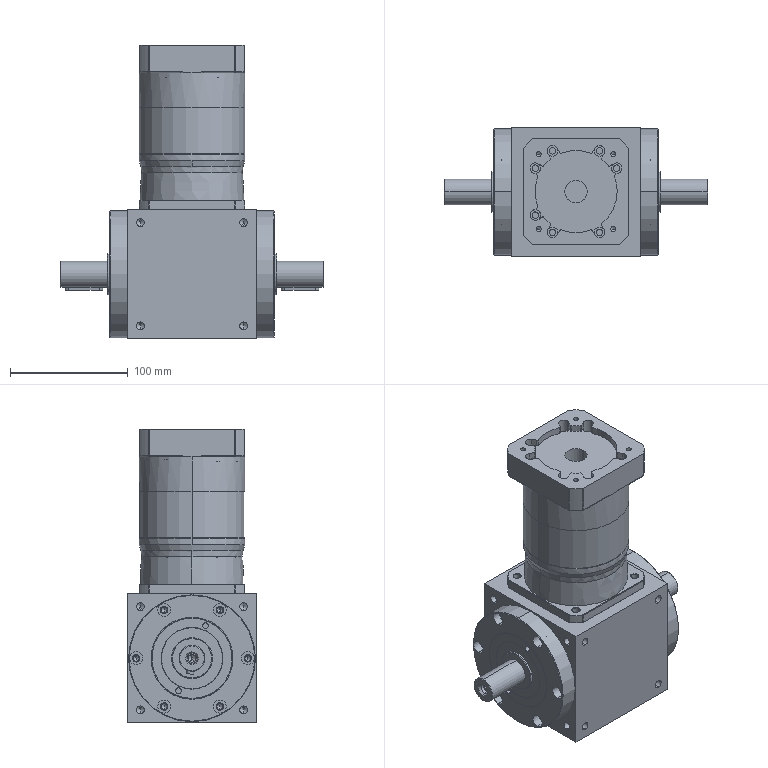Part | SolidWorks | features BaseBody 14 | 14 solids | 1605 faces | box 224 x 110 x 250 mm | volume 1662624 mm3 | cylinder 646 | spline 434 | cone 302 | plane 223 | commonest cylinder face diameters 65.21 x109 6.8 x84 4 x58 2 x42 5 x40 3 x24